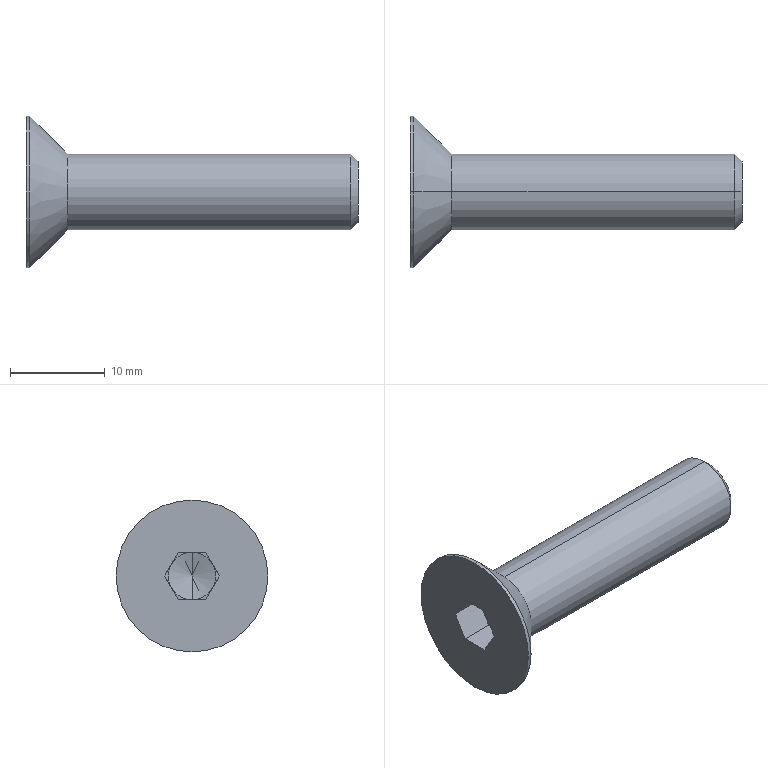Part | SolidWorks | features BaseBody 1 | 1 solid | 24 faces | box 35 x 16 x 16 mm | volume 2000 mm3 | plane 14 | cone 6 | cylinder 4 | commonest cylinder face diameters 8 x2 16 x2
STEP:
#1=CARTESIAN_POINT('',(0.,-1.443,-2.5));
#2=VERTEX_POINT('',#1);
#3=CARTESIAN_POINT('',(0.,-2.887,0.));
#4=VERTEX_POINT('',#3);
#5=CARTESIAN_POINT('',(0.,-1.443,-2.5));
#6=DIRECTION('',(0.,-0.5,0.866));
#7=VECTOR('',#6,1000.);
#8=LINE('',#5,#7);
#9=EDGE_CURVE('',#2,#4,#8,.T.);
#10=ORIENTED_EDGE('',*,*,#9,.F.);
#11=CARTESIAN_POINT('',(0.,1.443,-2.5));
#12=VERTEX_POINT('',#11);
#13=CARTESIAN_POINT('',(0.,-1.443,-2.5));
#14=DIRECTION('',(0.,1.,0.));
#15=VECTOR('',#14,1000.);
#16=LINE('',#13,#15);
#17=EDGE_CURVE('',#2,#12,#16,.T.);
#18=ORIENTED_EDGE('',*,*,#17,.T.);
#19=CARTESIAN_POINT('',(0.,2.887,0.));
#20=VERTEX_POINT('',#19);
#21=CARTESIAN_POINT('',(0.,2.887,0.));
#22=DIRECTION('',(0.,-0.5,-0.866));
#23=VECTOR('',#22,1000.);
#24=LINE('',#21,#23);
#25=EDGE_CURVE('',#20,#12,#24,.T.);
#26=ORIENTED_EDGE('',*,*,#25,.F.);
#27=CARTESIAN_POINT('',(0.,1.443,2.5));
#28=VERTEX_POINT('',#27);
#29=CARTESIAN_POINT('',(0.,1.443,2.5));
#30=DIRECTION('',(0.,0.5,-0.866));
#31=VECTOR('',#30,1000.);
#32=LINE('',#29,#31);
#33=EDGE_CURVE('',#28,#20,#32,.T.);
#34=ORIENTED_EDGE('',*,*,#33,.F.);
#35=CARTESIAN_POINT('',(0.,-1.443,2.5));
#36=VERTEX_POINT('',#35);
#37=CARTESIAN_POINT('',(0.,1.443,2.5));
#38=DIRECTION('',(0.,-1.,0.));
#39=VECTOR('',#38,1000.);
#40=LINE('',#37,#39);
#41=EDGE_CURVE('',#28,#36,#40,.T.);
#42=ORIENTED_EDGE('',*,*,#41,.T.);
#43=CARTESIAN_POINT('',(0.,-2.887,0.));
#44=DIRECTION('',(0.,0.5,0.866));
#45=VECTOR('',#44,1000.);
#46=LINE('',#43,#45);
#47=EDGE_CURVE('',#4,#36,#46,.T.);
#48=ORIENTED_EDGE('',*,*,#47,.F.);
#49=EDGE_LOOP('',(#10,#18,#26,#34,#42,#48));
#50=FACE_BOUND('',#49,.T.);
#51=CARTESIAN_POINT('',(0.,0.,-8.));
#52=VERTEX_POINT('',#51);
#53=CARTESIAN_POINT('',(0.,0.,8.));
#54=VERTEX_POINT('',#53);
#55=CARTESIAN_POINT('',(0.,0.,0.));
#56=DIRECTION('',(1.,0.,0.));
#57=DIRECTION('',(0.,0.,-1.));
#58=AXIS2_PLACEMENT_3D('',#55,#56,#57);
#59=CIRCLE('',#58,8.);
#60=EDGE_CURVE('',#52,#54,#59,.T.);
#61=ORIENTED_EDGE('',*,*,#60,.F.);
#62=CARTESIAN_POINT('',(0.,0.,0.));
#63=DIRECTION('',(1.,0.,0.));
#64=DIRECTION('',(0.,0.,1.));
#65=AXIS2_PLACEMENT_3D('',#62,#63,#64);
#66=CIRCLE('',#65,8.);
#67=EDGE_CURVE('',#54,#52,#66,.T.);
#68=ORIENTED_EDGE('',*,*,#67,.F.);
#69=EDGE_LOOP('',(#61,#68));
#70=FACE_OUTER_BOUND('',#69,.T.);
#71=CARTESIAN_POINT('',(0.,0.,0.));
#72=DIRECTION('',(1.,0.,0.));
#73=DIRECTION('',(0.,1.,0.));
#74=AXIS2_PLACEMENT_3D('',#71,#72,#73);
#75=PLANE('',#74);
#76=ADVANCED_FACE('',(#50,#70),#75,.F.);
#77=CARTESIAN_POINT('',(0.4,0.,-8.));
#78=VERTEX_POINT('',#77);
#79=CARTESIAN_POINT('',(0.,0.,-8.));
#80=DIRECTION('',(1.,0.,0.));
#81=VECTOR('',#80,1000.);
#82=LINE('',#79,#81);
#83=EDGE_CURVE('',#52,#78,#82,.T.);
#84=ORIENTED_EDGE('',*,*,#83,.T.);
#85=CARTESIAN_POINT('',(0.4,0.,8.));
#86=VERTEX_POINT('',#85);
#87=CARTESIAN_POINT('',(0.4,0.,0.));
#88=DIRECTION('',(-1.,0.,0.));
#89=DIRECTION('',(0.,0.,-1.));
#90=AXIS2_PLACEMENT_3D('',#87,#88,#89);
#91=CIRCLE('',#90,8.);
#92=EDGE_CURVE('',#78,#86,#91,.T.);
#93=ORIENTED_EDGE('',*,*,#92,.T.);
#94=CARTESIAN_POINT('',(0.,0.,8.));
#95=DIRECTION('',(1.,0.,0.));
#96=VECTOR('',#95,1000.);
#97=LINE('',#94,#96);
#98=EDGE_CURVE('',#54,#86,#97,.T.);
#99=ORIENTED_EDGE('',*,*,#98,.F.);
#100=ORIENTED_EDGE('',*,*,#67,.T.);
#101=EDGE_LOOP('',(#84,#93,#99,#100));
#102=FACE_OUTER_BOUND('',#101,.T.);
#103=CARTESIAN_POINT('',(35.,0.,0.));
#104=DIRECTION('',(-1.,0.,0.));
#105=DIRECTION('',(0.,0.,-1.));
#106=AXIS2_PLACEMENT_3D('',#103,#104,#105);
#107=CYLINDRICAL_SURFACE('',#106,8.);
#108=ADVANCED_FACE('',(#102),#107,.T.);
#109=ORIENTED_EDGE('',*,*,#98,.T.);
#110=CARTESIAN_POINT('',(0.4,0.,0.));
#111=DIRECTION('',(-1.,0.,0.));
#112=DIRECTION('',(0.,0.,1.));
#113=AXIS2_PLACEMENT_3D('',#110,#111,#112);
#114=CIRCLE('',#113,8.);
#115=EDGE_CURVE('',#86,#78,#114,.T.);
#116=ORIENTED_EDGE('',*,*,#115,.T.);
#117=ORIENTED_EDGE('',*,*,#83,.F.);
#118=ORIENTED_EDGE('',*,*,#60,.T.);
#119=EDGE_LOOP('',(#109,#116,#117,#118));
#120=FACE_OUTER_BOUND('',#119,.T.);
#121=CARTESIAN_POINT('',(35.,0.,0.));
#122=DIRECTION('',(-1.,0.,0.));
#123=DIRECTION('',(0.,0.,-1.));
#124=AXIS2_PLACEMENT_3D('',#121,#122,#123);
#125=CYLINDRICAL_SURFACE('',#124,8.);
#126=ADVANCED_FACE('',(#120),#125,.T.);
#127=CARTESIAN_POINT('',(4.4,0.,4.));
#128=VERTEX_POINT('',#127);
#129=CARTESIAN_POINT('',(0.4,0.,8.));
#130=DIRECTION('',(0.7071,0.,-0.7071));
#131=VECTOR('',#130,1000.);
#132=LINE('',#129,#131);
#133=EDGE_CURVE('',#86,#128,#132,.T.);
#134=ORIENTED_EDGE('',*,*,#133,.T.);
#135=CARTESIAN_POINT('',(4.4,0.,-4.));
#136=VERTEX_POINT('',#135);
#137=CARTESIAN_POINT('',(4.4,0.,0.));
#138=DIRECTION('',(1.,0.,0.));
#139=DIRECTION('',(0.,0.,-1.));
#140=AXIS2_PLACEMENT_3D('',#137,#138,#139);
#141=CIRCLE('',#140,4.);
#142=EDGE_CURVE('',#136,#128,#141,.T.);
#143=ORIENTED_EDGE('',*,*,#142,.F.);
#144=CARTESIAN_POINT('',(0.4,0.,-8.));
#145=DIRECTION('',(0.7071,0.,0.7071));
#146=VECTOR('',#145,1000.);
#147=LINE('',#144,#146);
#148=EDGE_CURVE('',#78,#136,#147,.T.);
#149=ORIENTED_EDGE('',*,*,#148,.F.);
#150=ORIENTED_EDGE('',*,*,#115,.F.);
#151=EDGE_LOOP('',(#134,#143,#149,#150));
#152=FACE_OUTER_BOUND('',#151,.T.);
#153=CARTESIAN_POINT('',(2.4,0.,0.));
#154=DIRECTION('',(-1.,0.,0.));
#155=DIRECTION('',(0.,0.,1.));
#156=AXIS2_PLACEMENT_3D('',#153,#154,#155);
#157=CONICAL_SURFACE('',#156,6.,0.7854);
#158=ADVANCED_FACE('',(#152),#157,.T.);
#159=ORIENTED_EDGE('',*,*,#148,.T.);
#160=CARTESIAN_POINT('',(4.4,0.,0.));
#161=DIRECTION('',(1.,0.,0.));
#162=DIRECTION('',(0.,0.,1.));
#163=AXIS2_PLACEMENT_3D('',#160,#161,#162);
#164=CIRCLE('',#163,4.);
#165=EDGE_CURVE('',#128,#136,#164,.T.);
#166=ORIENTED_EDGE('',*,*,#165,.F.);
#167=ORIENTED_EDGE('',*,*,#133,.F.);
#168=ORIENTED_EDGE('',*,*,#92,.F.);
#169=EDGE_LOOP('',(#159,#166,#167,#168));
#170=FACE_OUTER_BOUND('',#169,.T.);
#171=CARTESIAN_POINT('',(2.4,0.,0.));
#172=DIRECTION('',(-1.,0.,0.));
#173=DIRECTION('',(0.,0.,1.));
#174=AXIS2_PLACEMENT_3D('',#171,#172,#173);
#175=CONICAL_SURFACE('',#174,6.,0.7854);
#176=ADVANCED_FACE('',(#170),#175,.T.);
#177=CARTESIAN_POINT('',(34.233,0.,-4.));
#178=VERTEX_POINT('',#177);
#179=CARTESIAN_POINT('',(4.4,0.,-4.));
#180=DIRECTION('',(1.,0.,0.));
#181=VECTOR('',#180,1000.);
#182=LINE('',#179,#181);
#183=EDGE_CURVE('',#136,#178,#182,.T.);
#184=ORIENTED_EDGE('',*,*,#183,.T.);
#185=CARTESIAN_POINT('',(34.233,0.,4.));
#186=VERTEX_POINT('',#185);
#187=CARTESIAN_POINT('',(34.233,0.,0.));
#188=DIRECTION('',(-1.,0.,0.));
#189=DIRECTION('',(0.,0.,-1.));
#190=AXIS2_PLACEMENT_3D('',#187,#188,#189);
#191=CIRCLE('',#190,4.);
#192=EDGE_CURVE('',#178,#186,#191,.T.);
#193=ORIENTED_EDGE('',*,*,#192,.T.);
#194=CARTESIAN_POINT('',(4.4,0.,4.));
#195=DIRECTION('',(1.,0.,0.));
#196=VECTOR('',#195,1000.);
#197=LINE('',#194,#196);
#198=EDGE_CURVE('',#128,#186,#197,.T.);
#199=ORIENTED_EDGE('',*,*,#198,.F.);
#200=ORIENTED_EDGE('',*,*,#165,.T.);
#201=EDGE_LOOP('',(#184,#193,#199,#200));
#202=FACE_OUTER_BOUND('',#201,.T.);
#203=CARTESIAN_POINT('',(35.,0.,0.));
#204=DIRECTION('',(-1.,0.,0.));
#205=DIRECTION('',(0.,0.,-1.));
#206=AXIS2_PLACEMENT_3D('',#203,#204,#205);
#207=CYLINDRICAL_SURFACE('',#206,4.);
#208=ADVANCED_FACE('',(#202),#207,.T.);
#209=ORIENTED_EDGE('',*,*,#198,.T.);
#210=CARTESIAN_POINT('',(34.233,0.,0.));
#211=DIRECTION('',(-1.,0.,0.));
#212=DIRECTION('',(0.,0.,1.));
#213=AXIS2_PLACEMENT_3D('',#210,#211,#212);
#214=CIRCLE('',#213,4.);
#215=EDGE_CURVE('',#186,#178,#214,.T.);
#216=ORIENTED_EDGE('',*,*,#215,.T.);
#217=ORIENTED_EDGE('',*,*,#183,.F.);
#218=ORIENTED_EDGE('',*,*,#142,.T.);
#219=EDGE_LOOP('',(#209,#216,#217,#218));
#220=FACE_OUTER_BOUND('',#219,.T.);
#221=CARTESIAN_POINT('',(35.,0.,0.));
#222=DIRECTION('',(-1.,0.,0.));
#223=DIRECTION('',(0.,0.,-1.));
#224=AXIS2_PLACEMENT_3D('',#221,#222,#223);
#225=CYLINDRICAL_SURFACE('',#224,4.);
#226=ADVANCED_FACE('',(#220),#225,.T.);
#227=CARTESIAN_POINT('',(35.,0.,3.233));
#228=VERTEX_POINT('',#227);
#229=CARTESIAN_POINT('',(34.233,0.,4.));
#230=DIRECTION('',(0.7071,0.,-0.7071));
#231=VECTOR('',#230,1000.);
#232=LINE('',#229,#231);
#233=EDGE_CURVE('',#186,#228,#232,.T.);
#234=ORIENTED_EDGE('',*,*,#233,.T.);
#235=CARTESIAN_POINT('',(35.,0.,-3.233));
#236=VERTEX_POINT('',#235);
#237=CARTESIAN_POINT('',(35.,0.,0.));
#238=DIRECTION('',(-1.,0.,0.));
#239=DIRECTION('',(0.,0.,1.));
#240=AXIS2_PLACEMENT_3D('',#237,#238,#239);
#241=CIRCLE('',#240,3.233);
#242=EDGE_CURVE('',#228,#236,#241,.T.);
#243=ORIENTED_EDGE('',*,*,#242,.T.);
#244=CARTESIAN_POINT('',(34.233,0.,-4.));
#245=DIRECTION('',(0.7071,0.,0.7071));
#246=VECTOR('',#245,1000.);
#247=LINE('',#244,#246);
#248=EDGE_CURVE('',#178,#236,#247,.T.);
#249=ORIENTED_EDGE('',*,*,#248,.F.);
#250=ORIENTED_EDGE('',*,*,#215,.F.);
#251=EDGE_LOOP('',(#234,#243,#249,#250));
#252=FACE_OUTER_BOUND('',#251,.T.);
#253=CARTESIAN_POINT('',(34.617,0.,0.));
#254=DIRECTION('',(-1.,0.,0.));
#255=DIRECTION('',(0.,0.,1.));
#256=AXIS2_PLACEMENT_3D('',#253,#254,#255);
#257=CONICAL_SURFACE('',#256,3.616,0.7854);
#258=ADVANCED_FACE('',(#252),#257,.T.);
#259=ORIENTED_EDGE('',*,*,#248,.T.);
#260=CARTESIAN_POINT('',(35.,0.,0.));
#261=DIRECTION('',(-1.,0.,0.));
#262=DIRECTION('',(0.,0.,-1.));
#263=AXIS2_PLACEMENT_3D('',#260,#261,#262);
#264=CIRCLE('',#263,3.233);
#265=EDGE_CURVE('',#236,#228,#264,.T.);
#266=ORIENTED_EDGE('',*,*,#265,.T.);
#267=ORIENTED_EDGE('',*,*,#233,.F.);
#268=ORIENTED_EDGE('',*,*,#192,.F.);
#269=EDGE_LOOP('',(#259,#266,#267,#268));
#270=FACE_OUTER_BOUND('',#269,.T.);
#271=CARTESIAN_POINT('',(34.617,0.,0.));
#272=DIRECTION('',(-1.,0.,0.));
#273=DIRECTION('',(0.,0.,1.));
#274=AXIS2_PLACEMENT_3D('',#271,#272,#273);
#275=CONICAL_SURFACE('',#274,3.616,0.7854);
#276=ADVANCED_FACE('',(#270),#275,.T.);
#277=ORIENTED_EDGE('',*,*,#265,.F.);
#278=ORIENTED_EDGE('',*,*,#242,.F.);
#279=EDGE_LOOP('',(#277,#278));
#280=FACE_OUTER_BOUND('',#279,.T.);
#281=CARTESIAN_POINT('',(35.,3.233,0.));
#282=DIRECTION('',(-1.,0.,0.));
#283=DIRECTION('',(0.,0.,1.));
#284=AXIS2_PLACEMENT_3D('',#281,#282,#283);
#285=PLANE('',#284);
#286=ADVANCED_FACE('',(#280),#285,.F.);
#287=CARTESIAN_POINT('',(3.52,-1.443,2.5));
#288=VERTEX_POINT('',#287);
#289=CARTESIAN_POINT('',(3.52,-1.443,2.5));
#290=DIRECTION('',(-1.,0.,0.));
#291=VECTOR('',#290,1000.);
#292=LINE('',#289,#291);
#293=EDGE_CURVE('',#288,#36,#292,.T.);
#294=ORIENTED_EDGE('',*,*,#293,.F.);
#295=CARTESIAN_POINT('',(3.52,-2.165,1.25));
#296=VERTEX_POINT('',#295);
#297=CARTESIAN_POINT('',(3.52,-1.443,2.5));
#298=DIRECTION('',(0.,-0.5,-0.866));
#299=VECTOR('',#298,1000.);
#300=LINE('',#297,#299);
#301=EDGE_CURVE('',#288,#296,#300,.T.);
#302=ORIENTED_EDGE('',*,*,#301,.T.);
#303=CARTESIAN_POINT('',(3.52,-2.887,0.));
#304=VERTEX_POINT('',#303);
#305=CARTESIAN_POINT('',(3.52,-2.165,1.25));
#306=DIRECTION('',(0.,-0.5,-0.866));
#307=VECTOR('',#306,1000.);
#308=LINE('',#305,#307);
#309=EDGE_CURVE('',#296,#304,#308,.T.);
#310=ORIENTED_EDGE('',*,*,#309,.T.);
#311=CARTESIAN_POINT('',(3.52,-2.887,0.));
#312=DIRECTION('',(-1.,0.,0.));
#313=VECTOR('',#312,1000.);
#314=LINE('',#311,#313);
#315=EDGE_CURVE('',#304,#4,#314,.T.);
#316=ORIENTED_EDGE('',*,*,#315,.T.);
#317=ORIENTED_EDGE('',*,*,#47,.T.);
#318=EDGE_LOOP('',(#294,#302,#310,#316,#317));
#319=FACE_OUTER_BOUND('',#318,.T.);
#320=CARTESIAN_POINT('',(3.52,-1.443,2.5));
#321=DIRECTION('',(0.,0.866,-0.5));
#322=DIRECTION('',(-1.,0.,0.));
#323=AXIS2_PLACEMENT_3D('',#320,#321,#322);
#324=PLANE('',#323);
#325=ADVANCED_FACE('',(#319),#324,.T.);
#326=ORIENTED_EDGE('',*,*,#315,.F.);
#327=CARTESIAN_POINT('',(3.52,-2.165,-1.25));
#328=VERTEX_POINT('',#327);
#329=CARTESIAN_POINT('',(3.52,-2.887,0.));
#330=DIRECTION('',(0.,0.5,-0.866));
#331=VECTOR('',#330,1000.);
#332=LINE('',#329,#331);
#333=EDGE_CURVE('',#304,#328,#332,.T.);
#334=ORIENTED_EDGE('',*,*,#333,.T.);
#335=CARTESIAN_POINT('',(3.52,-1.443,-2.5));
#336=VERTEX_POINT('',#335);
#337=CARTESIAN_POINT('',(3.52,-2.165,-1.25));
#338=DIRECTION('',(0.,0.5,-0.866));
#339=VECTOR('',#338,1000.);
#340=LINE('',#337,#339);
#341=EDGE_CURVE('',#328,#336,#340,.T.);
#342=ORIENTED_EDGE('',*,*,#341,.T.);
#343=CARTESIAN_POINT('',(3.52,-1.443,-2.5));
#344=DIRECTION('',(-1.,0.,0.));
#345=VECTOR('',#344,1000.);
#346=LINE('',#343,#345);
#347=EDGE_CURVE('',#336,#2,#346,.T.);
#348=ORIENTED_EDGE('',*,*,#347,.T.);
#349=ORIENTED_EDGE('',*,*,#9,.T.);
#350=EDGE_LOOP('',(#326,#334,#342,#348,#349));
#351=FACE_OUTER_BOUND('',#350,.T.);
#352=CARTESIAN_POINT('',(3.52,-2.887,0.));
#353=DIRECTION('',(0.,0.866,0.5));
#354=DIRECTION('',(1.,0.,0.));
#355=AXIS2_PLACEMENT_3D('',#352,#353,#354);
#356=PLANE('',#355);
#357=ADVANCED_FACE('',(#351),#356,.T.);
#358=ORIENTED_EDGE('',*,*,#347,.F.);
#359=CARTESIAN_POINT('',(3.52,0.,-2.5));
#360=VERTEX_POINT('',#359);
#361=CARTESIAN_POINT('',(3.52,-1.443,-2.5));
#362=DIRECTION('',(0.,1.,0.));
#363=VECTOR('',#362,1000.);
#364=LINE('',#361,#363);
#365=EDGE_CURVE('',#336,#360,#364,.T.);
#366=ORIENTED_EDGE('',*,*,#365,.T.);
#367=CARTESIAN_POINT('',(3.52,1.443,-2.5));
#368=VERTEX_POINT('',#367);
#369=CARTESIAN_POINT('',(3.52,0.,-2.5));
#370=DIRECTION('',(0.,1.,0.));
#371=VECTOR('',#370,1000.);
#372=LINE('',#369,#371);
#373=EDGE_CURVE('',#360,#368,#372,.T.);
#374=ORIENTED_EDGE('',*,*,#373,.T.);
#375=CARTESIAN_POINT('',(3.52,1.443,-2.5));
#376=DIRECTION('',(-1.,0.,0.));
#377=VECTOR('',#376,1000.);
#378=LINE('',#375,#377);
#379=EDGE_CURVE('',#368,#12,#378,.T.);
#380=ORIENTED_EDGE('',*,*,#379,.T.);
#381=ORIENTED_EDGE('',*,*,#17,.F.);
#382=EDGE_LOOP('',(#358,#366,#374,#380,#381));
#383=FACE_OUTER_BOUND('',#382,.T.);
#384=CARTESIAN_POINT('',(3.52,-1.443,-2.5));
#385=DIRECTION('',(0.,0.,1.));
#386=DIRECTION('',(1.,0.,0.));
#387=AXIS2_PLACEMENT_3D('',#384,#385,#386);
#388=PLANE('',#387);
#389=ADVANCED_FACE('',(#383),#388,.T.);
#390=ORIENTED_EDGE('',*,*,#379,.F.);
#391=CARTESIAN_POINT('',(3.52,2.165,-1.25));
#392=VERTEX_POINT('',#391);
#393=CARTESIAN_POINT('',(3.52,1.443,-2.5));
#394=DIRECTION('',(0.,0.5,0.866));
#395=VECTOR('',#394,1000.);
#396=LINE('',#393,#395);
#397=EDGE_CURVE('',#368,#392,#396,.T.);
#398=ORIENTED_EDGE('',*,*,#397,.T.);
#399=CARTESIAN_POINT('',(3.52,2.887,0.));
#400=VERTEX_POINT('',#399);
#401=CARTESIAN_POINT('',(3.52,2.165,-1.25));
#402=DIRECTION('',(0.,0.5,0.866));
#403=VECTOR('',#402,1000.);
#404=LINE('',#401,#403);
#405=EDGE_CURVE('',#392,#400,#404,.T.);
#406=ORIENTED_EDGE('',*,*,#405,.T.);
#407=CARTESIAN_POINT('',(3.52,2.887,0.));
#408=DIRECTION('',(-1.,0.,0.));
#409=VECTOR('',#408,1000.);
#410=LINE('',#407,#409);
#411=EDGE_CURVE('',#400,#20,#410,.T.);
#412=ORIENTED_EDGE('',*,*,#411,.T.);
#413=ORIENTED_EDGE('',*,*,#25,.T.);
#414=EDGE_LOOP('',(#390,#398,#406,#412,#413));
#415=FACE_OUTER_BOUND('',#414,.T.);
#416=CARTESIAN_POINT('',(3.52,1.443,-2.5));
#417=DIRECTION('',(0.,-0.866,0.5));
#418=DIRECTION('',(-1.,0.,0.));
#419=AXIS2_PLACEMENT_3D('',#416,#417,#418);
#420=PLANE('',#419);
#421=ADVANCED_FACE('',(#415),#420,.T.);
#422=ORIENTED_EDGE('',*,*,#411,.F.);
#423=CARTESIAN_POINT('',(3.52,2.165,1.25));
#424=VERTEX_POINT('',#423);
#425=CARTESIAN_POINT('',(3.52,2.887,0.));
#426=DIRECTION('',(0.,-0.5,0.866));
#427=VECTOR('',#426,1000.);
#428=LINE('',#425,#427);
#429=EDGE_CURVE('',#400,#424,#428,.T.);
#430=ORIENTED_EDGE('',*,*,#429,.T.);
#431=CARTESIAN_POINT('',(3.52,1.443,2.5));
#432=VERTEX_POINT('',#431);
#433=CARTESIAN_POINT('',(3.52,2.165,1.25));
#434=DIRECTION('',(0.,-0.5,0.866));
#435=VECTOR('',#434,1000.);
#436=LINE('',#433,#435);
#437=EDGE_CURVE('',#424,#432,#436,.T.);
#438=ORIENTED_EDGE('',*,*,#437,.T.);
#439=CARTESIAN_POINT('',(3.52,1.443,2.5));
#440=DIRECTION('',(-1.,0.,0.));
#441=VECTOR('',#440,1000.);
#442=LINE('',#439,#441);
#443=EDGE_CURVE('',#432,#28,#442,.T.);
#444=ORIENTED_EDGE('',*,*,#443,.T.);
#445=ORIENTED_EDGE('',*,*,#33,.T.);
#446=EDGE_LOOP('',(#422,#430,#438,#444,#445));
#447=FACE_OUTER_BOUND('',#446,.T.);
#448=CARTESIAN_POINT('',(3.52,2.887,0.));
#449=DIRECTION('',(0.,-0.866,-0.5));
#450=DIRECTION('',(0.,0.5,-0.866));
#451=AXIS2_PLACEMENT_3D('',#448,#449,#450);
#452=PLANE('',#451);
#453=ADVANCED_FACE('',(#447),#452,.T.);
#454=ORIENTED_EDGE('',*,*,#443,.F.);
#455=CARTESIAN_POINT('',(3.52,0.,2.5));
#456=VERTEX_POINT('',#455);
#457=CARTESIAN_POINT('',(3.52,1.443,2.5));
#458=DIRECTION('',(0.,-1.,0.));
#459=VECTOR('',#458,1000.);
#460=LINE('',#457,#459);
#461=EDGE_CURVE('',#432,#456,#460,.T.);
#462=ORIENTED_EDGE('',*,*,#461,.T.);
#463=CARTESIAN_POINT('',(3.52,0.,2.5));
#464=DIRECTION('',(0.,-1.,0.));
#465=VECTOR('',#464,1000.);
#466=LINE('',#463,#465);
#467=EDGE_CURVE('',#456,#288,#466,.T.);
#468=ORIENTED_EDGE('',*,*,#467,.T.);
#469=ORIENTED_EDGE('',*,*,#293,.T.);
#470=ORIENTED_EDGE('',*,*,#41,.F.);
#471=EDGE_LOOP('',(#454,#462,#468,#469,#470));
#472=FACE_OUTER_BOUND('',#471,.T.);
#473=CARTESIAN_POINT('',(3.52,1.443,2.5));
#474=DIRECTION('',(0.,0.,-1.));
#475=DIRECTION('',(0.,-1.,0.));
#476=AXIS2_PLACEMENT_3D('',#473,#474,#475);
#477=PLANE('',#476);
#478=ADVANCED_FACE('',(#472),#477,.T.);
#479=ORIENTED_EDGE('',*,*,#301,.F.);
#480=ORIENTED_EDGE('',*,*,#467,.F.);
#481=CARTESIAN_POINT('',(3.52,0.,0.));
#482=DIRECTION('',(-1.,0.,0.));
#483=DIRECTION('',(0.,-0.866,0.5));
#484=AXIS2_PLACEMENT_3D('',#481,#482,#483);
#485=CIRCLE('',#484,2.5);
#486=EDGE_CURVE('',#296,#456,#485,.T.);
#487=ORIENTED_EDGE('',*,*,#486,.F.);
#488=EDGE_LOOP('',(#479,#480,#487));
#489=FACE_OUTER_BOUND('',#488,.T.);
#490=CARTESIAN_POINT('',(3.52,0.,0.));
#491=DIRECTION('',(1.,0.,0.));
#492=DIRECTION('',(0.,1.,0.));
#493=AXIS2_PLACEMENT_3D('',#490,#491,#492);
#494=PLANE('',#493);
#495=ADVANCED_FACE('',(#489),#494,.F.);
#496=CARTESIAN_POINT('',(3.52,0.,0.));
#497=DIRECTION('',(-1.,0.,0.));
#498=DIRECTION('',(0.,-0.866,-0.5));
#499=AXIS2_PLACEMENT_3D('',#496,#497,#498);
#500=CIRCLE('',#499,2.5);
#501=EDGE_CURVE('',#328,#296,#500,.T.);
#502=ORIENTED_EDGE('',*,*,#501,.T.);
#503=ORIENTED_EDGE('',*,*,#486,.T.);
#504=CARTESIAN_POINT('',(4.19,0.,0.));
#505=VERTEX_POINT('',#504);
#506=CARTESIAN_POINT('',(3.52,0.,2.5));
#507=DIRECTION('',(0.2588,0.,-0.9659));
#508=VECTOR('',#507,1000.);
#509=LINE('',#506,#508);
#510=EDGE_CURVE('',#456,#505,#509,.T.);
#511=ORIENTED_EDGE('',*,*,#510,.T.);
#512=CARTESIAN_POINT('',(3.52,0.,-2.5));
#513=DIRECTION('',(0.2588,0.,0.9659));
#514=VECTOR('',#513,1000.);
#515=LINE('',#512,#514);
#516=EDGE_CURVE('',#360,#505,#515,.T.);
#517=ORIENTED_EDGE('',*,*,#516,.F.);
#518=CARTESIAN_POINT('',(3.52,0.,0.));
#519=DIRECTION('',(-1.,0.,0.));
#520=DIRECTION('',(0.,0.,-1.));
#521=AXIS2_PLACEMENT_3D('',#518,#519,#520);
#522=CIRCLE('',#521,2.5);
#523=EDGE_CURVE('',#360,#328,#522,.T.);
#524=ORIENTED_EDGE('',*,*,#523,.T.);
#525=EDGE_LOOP('',(#502,#503,#511,#517,#524));
#526=FACE_OUTER_BOUND('',#525,.T.);
#527=CARTESIAN_POINT('',(3.839,0.,0.));
#528=DIRECTION('',(-1.,0.,0.));
#529=DIRECTION('',(0.,0.,1.));
#530=AXIS2_PLACEMENT_3D('',#527,#528,#529);
#531=CONICAL_SURFACE('',#530,1.308,1.309);
#532=ADVANCED_FACE('',(#526),#531,.F.);
#533=ORIENTED_EDGE('',*,*,#365,.F.);
#534=ORIENTED_EDGE('',*,*,#341,.F.);
#535=ORIENTED_EDGE('',*,*,#523,.F.);
#536=EDGE_LOOP('',(#533,#534,#535));
#537=FACE_OUTER_BOUND('',#536,.T.);
#538=CARTESIAN_POINT('',(3.52,0.,0.));
#539=DIRECTION('',(1.,0.,0.));
#540=DIRECTION('',(0.,1.,0.));
#541=AXIS2_PLACEMENT_3D('',#538,#539,#540);
#542=PLANE('',#541);
#543=ADVANCED_FACE('',(#537),#542,.F.);
#544=CARTESIAN_POINT('',(3.52,0.,0.));
#545=DIRECTION('',(-1.,0.,0.));
#546=DIRECTION('',(0.,0.866,-0.5));
#547=AXIS2_PLACEMENT_3D('',#544,#545,#546);
#548=CIRCLE('',#547,2.5);
#549=EDGE_CURVE('',#392,#360,#548,.T.);
#550=ORIENTED_EDGE('',*,*,#549,.T.);
#551=ORIENTED_EDGE('',*,*,#516,.T.);
#552=ORIENTED_EDGE('',*,*,#510,.F.);
#553=CARTESIAN_POINT('',(3.52,0.,0.));
#554=DIRECTION('',(-1.,0.,0.));
#555=DIRECTION('',(0.,0.,1.));
#556=AXIS2_PLACEMENT_3D('',#553,#554,#555);
#557=CIRCLE('',#556,2.5);
#558=EDGE_CURVE('',#456,#424,#557,.T.);
#559=ORIENTED_EDGE('',*,*,#558,.T.);
#560=CARTESIAN_POINT('',(3.52,0.,0.));
#561=DIRECTION('',(-1.,0.,0.));
#562=DIRECTION('',(0.,0.866,0.5));
#563=AXIS2_PLACEMENT_3D('',#560,#561,#562);
#564=CIRCLE('',#563,2.5);
#565=EDGE_CURVE('',#424,#392,#564,.T.);
#566=ORIENTED_EDGE('',*,*,#565,.T.);
#567=EDGE_LOOP('',(#550,#551,#552,#559,#566));
#568=FACE_OUTER_BOUND('',#567,.T.);
#569=CARTESIAN_POINT('',(3.839,0.,0.));
#570=DIRECTION('',(-1.,0.,0.));
#571=DIRECTION('',(0.,0.,1.));
#572=AXIS2_PLACEMENT_3D('',#569,#570,#571);
#573=CONICAL_SURFACE('',#572,1.308,1.309);
#574=ADVANCED_FACE('',(#568),#573,.F.);
#575=ORIENTED_EDGE('',*,*,#565,.F.);
#576=ORIENTED_EDGE('',*,*,#429,.F.);
#577=ORIENTED_EDGE('',*,*,#405,.F.);
#578=EDGE_LOOP('',(#575,#576,#577));
#579=FACE_OUTER_BOUND('',#578,.T.);
#580=CARTESIAN_POINT('',(3.52,0.,0.));
#581=DIRECTION('',(1.,0.,0.));
#582=DIRECTION('',(0.,1.,0.));
#583=AXIS2_PLACEMENT_3D('',#580,#581,#582);
#584=PLANE('',#583);
#585=ADVANCED_FACE('',(#579),#584,.F.);
#586=ORIENTED_EDGE('',*,*,#461,.F.);
#587=ORIENTED_EDGE('',*,*,#437,.F.);
#588=ORIENTED_EDGE('',*,*,#558,.F.);
#589=EDGE_LOOP('',(#586,#587,#588));
#590=FACE_OUTER_BOUND('',#589,.T.);
#591=CARTESIAN_POINT('',(3.52,0.,0.));
#592=DIRECTION('',(1.,0.,0.));
#593=DIRECTION('',(0.,1.,0.));
#594=AXIS2_PLACEMENT_3D('',#591,#592,#593);
#595=PLANE('',#594);
#596=ADVANCED_FACE('',(#590),#595,.F.);
#597=ORIENTED_EDGE('',*,*,#397,.F.);
#598=ORIENTED_EDGE('',*,*,#373,.F.);
#599=ORIENTED_EDGE('',*,*,#549,.F.);
#600=EDGE_LOOP('',(#597,#598,#599));
#601=FACE_OUTER_BOUND('',#600,.T.);
#602=CARTESIAN_POINT('',(3.52,0.,0.));
#603=DIRECTION('',(1.,0.,0.));
#604=DIRECTION('',(0.,1.,0.));
#605=AXIS2_PLACEMENT_3D('',#602,#603,#604);
#606=PLANE('',#605);
#607=ADVANCED_FACE('',(#601),#606,.F.);
#608=ORIENTED_EDGE('',*,*,#333,.F.);
#609=ORIENTED_EDGE('',*,*,#309,.F.);
#610=ORIENTED_EDGE('',*,*,#501,.F.);
#611=EDGE_LOOP('',(#608,#609,#610));
#612=FACE_OUTER_BOUND('',#611,.T.);
#613=CARTESIAN_POINT('',(3.52,0.,0.));
#614=DIRECTION('',(1.,0.,0.));
#615=DIRECTION('',(0.,1.,0.));
#616=AXIS2_PLACEMENT_3D('',#613,#614,#615);
#617=PLANE('',#616);
#618=ADVANCED_FACE('',(#612),#617,.F.);
#619=CLOSED_SHELL('',(#76,#108,#126,#158,#176,#208,#226,#258,#276,#286,#325,#357,#389,#421,#453,#478,#495,#532,#543,#574,#585,#596,#607,#618));
#620=MANIFOLD_SOLID_BREP('',#619);
#621=CARTESIAN_POINT('',(0.,0.,0.));
#622=DIRECTION('',(0.,0.,1.));
#623=DIRECTION('',(1.,0.,0.));
#624=AXIS2_PLACEMENT_3D('',#621,#622,#623);
#625=(LENGTH_UNIT()NAMED_UNIT(*)SI_UNIT(.MILLI.,.METRE.));
#626=UNCERTAINTY_MEASURE_WITH_UNIT(LENGTH_MEASURE(0.00001),#625,'','');
#627=(NAMED_UNIT(*)PLANE_ANGLE_UNIT()SI_UNIT($,.RADIAN.));
#628=(NAMED_UNIT(*)SI_UNIT($,.STERADIAN.)SOLID_ANGLE_UNIT());
#629=(GEOMETRIC_REPRESENTATION_CONTEXT(3)GLOBAL_UNCERTAINTY_ASSIGNED_CONTEXT((#626))GLOBAL_UNIT_ASSIGNED_CONTEXT((#625,#627,#628))REPRESENTATION_CONTEXT('',''));
#630=ADVANCED_BREP_SHAPE_REPRESENTATION('',(#620,#624),#629);